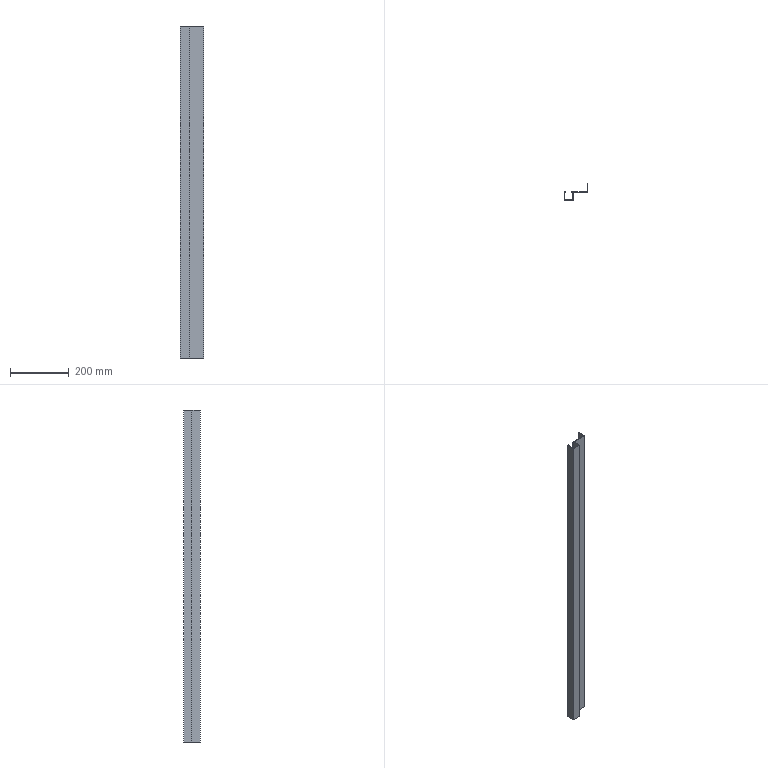Part | STEP file | Rieles_1-24 | 1 solid | 18 faces | box 81.4 x 57.7 x 1129 mm | volume 294161 mm3 | plane 18
STEP:
#1=CARTESIAN_POINT('',(10.,26.2,-677.));
#2=VERTEX_POINT('',#1);
#3=CARTESIAN_POINT('',(10.,27.7,-677.));
#4=VERTEX_POINT('',#3);
#5=CARTESIAN_POINT('',(10.,27.35,-677.));
#6=DIRECTION('',(0.,1.,0.));
#7=VECTOR('',#6,1000.);
#8=LINE('',#5,#7);
#9=EDGE_CURVE('',#2,#4,#8,.T.);
#10=ORIENTED_EDGE('',*,*,#9,.T.);
#11=CARTESIAN_POINT('',(64.2,27.7,-677.));
#12=VERTEX_POINT('',#11);
#13=CARTESIAN_POINT('',(25.,27.7,-677.));
#14=DIRECTION('',(1.,0.,0.));
#15=VECTOR('',#14,1000.);
#16=LINE('',#13,#15);
#17=EDGE_CURVE('',#4,#12,#16,.T.);
#18=ORIENTED_EDGE('',*,*,#17,.T.);
#19=CARTESIAN_POINT('',(64.2,56.2,-677.));
#20=VERTEX_POINT('',#19);
#21=CARTESIAN_POINT('',(64.2,27.35,-677.));
#22=DIRECTION('',(0.,1.,0.));
#23=VECTOR('',#22,1000.);
#24=LINE('',#21,#23);
#25=EDGE_CURVE('',#12,#20,#24,.T.);
#26=ORIENTED_EDGE('',*,*,#25,.T.);
#27=CARTESIAN_POINT('',(65.7,56.2,-677.));
#28=VERTEX_POINT('',#27);
#29=CARTESIAN_POINT('',(25.,56.2,-677.));
#30=DIRECTION('',(1.,0.,0.));
#31=VECTOR('',#30,1000.);
#32=LINE('',#29,#31);
#33=EDGE_CURVE('',#20,#28,#32,.T.);
#34=ORIENTED_EDGE('',*,*,#33,.T.);
#35=CARTESIAN_POINT('',(65.7,26.2,-677.));
#36=VERTEX_POINT('',#35);
#37=CARTESIAN_POINT('',(65.7,27.35,-677.));
#38=DIRECTION('',(0.,-1.,0.));
#39=VECTOR('',#38,1000.);
#40=LINE('',#37,#39);
#41=EDGE_CURVE('',#28,#36,#40,.T.);
#42=ORIENTED_EDGE('',*,*,#41,.T.);
#43=CARTESIAN_POINT('',(15.7,26.2,-677.));
#44=VERTEX_POINT('',#43);
#45=CARTESIAN_POINT('',(25.,26.2,-677.));
#46=DIRECTION('',(-1.,0.,0.));
#47=VECTOR('',#46,1000.);
#48=LINE('',#45,#47);
#49=EDGE_CURVE('',#36,#44,#48,.T.);
#50=ORIENTED_EDGE('',*,*,#49,.T.);
#51=CARTESIAN_POINT('',(15.7,-1.5,-677.));
#52=VERTEX_POINT('',#51);
#53=CARTESIAN_POINT('',(15.7,27.35,-677.));
#54=DIRECTION('',(0.,-1.,0.));
#55=VECTOR('',#54,1000.);
#56=LINE('',#53,#55);
#57=EDGE_CURVE('',#44,#52,#56,.T.);
#58=ORIENTED_EDGE('',*,*,#57,.T.);
#59=CARTESIAN_POINT('',(-15.7,-1.5,-677.));
#60=VERTEX_POINT('',#59);
#61=CARTESIAN_POINT('',(25.,-1.5,-677.));
#62=DIRECTION('',(-1.,0.,0.));
#63=VECTOR('',#62,1000.);
#64=LINE('',#61,#63);
#65=EDGE_CURVE('',#52,#60,#64,.T.);
#66=ORIENTED_EDGE('',*,*,#65,.T.);
#67=CARTESIAN_POINT('',(-15.7,27.7,-677.));
#68=VERTEX_POINT('',#67);
#69=CARTESIAN_POINT('',(-15.7,27.35,-677.));
#70=DIRECTION('',(0.,1.,0.));
#71=VECTOR('',#70,1000.);
#72=LINE('',#69,#71);
#73=EDGE_CURVE('',#60,#68,#72,.T.);
#74=ORIENTED_EDGE('',*,*,#73,.T.);
#75=CARTESIAN_POINT('',(-10.,27.7,-677.));
#76=VERTEX_POINT('',#75);
#77=CARTESIAN_POINT('',(25.,27.7,-677.));
#78=DIRECTION('',(1.,0.,0.));
#79=VECTOR('',#78,1000.);
#80=LINE('',#77,#79);
#81=EDGE_CURVE('',#68,#76,#80,.T.);
#82=ORIENTED_EDGE('',*,*,#81,.T.);
#83=CARTESIAN_POINT('',(-10.,26.2,-677.));
#84=VERTEX_POINT('',#83);
#85=CARTESIAN_POINT('',(-10.,27.35,-677.));
#86=DIRECTION('',(0.,-1.,0.));
#87=VECTOR('',#86,1000.);
#88=LINE('',#85,#87);
#89=EDGE_CURVE('',#76,#84,#88,.T.);
#90=ORIENTED_EDGE('',*,*,#89,.T.);
#91=CARTESIAN_POINT('',(-14.2,26.2,-677.));
#92=VERTEX_POINT('',#91);
#93=CARTESIAN_POINT('',(25.,26.2,-677.));
#94=DIRECTION('',(-1.,0.,0.));
#95=VECTOR('',#94,1000.);
#96=LINE('',#93,#95);
#97=EDGE_CURVE('',#84,#92,#96,.T.);
#98=ORIENTED_EDGE('',*,*,#97,.T.);
#99=CARTESIAN_POINT('',(-14.2,0.,-677.));
#100=VERTEX_POINT('',#99);
#101=CARTESIAN_POINT('',(-14.2,27.35,-677.));
#102=DIRECTION('',(0.,-1.,0.));
#103=VECTOR('',#102,1000.);
#104=LINE('',#101,#103);
#105=EDGE_CURVE('',#92,#100,#104,.T.);
#106=ORIENTED_EDGE('',*,*,#105,.T.);
#107=CARTESIAN_POINT('',(14.2,0.,-677.));
#108=VERTEX_POINT('',#107);
#109=CARTESIAN_POINT('',(25.,0.,-677.));
#110=DIRECTION('',(1.,0.,0.));
#111=VECTOR('',#110,1000.);
#112=LINE('',#109,#111);
#113=EDGE_CURVE('',#100,#108,#112,.T.);
#114=ORIENTED_EDGE('',*,*,#113,.T.);
#115=CARTESIAN_POINT('',(14.2,26.2,-677.));
#116=VERTEX_POINT('',#115);
#117=CARTESIAN_POINT('',(14.2,27.35,-677.));
#118=DIRECTION('',(0.,1.,0.));
#119=VECTOR('',#118,1000.);
#120=LINE('',#117,#119);
#121=EDGE_CURVE('',#108,#116,#120,.T.);
#122=ORIENTED_EDGE('',*,*,#121,.T.);
#123=CARTESIAN_POINT('',(25.,26.2,-677.));
#124=DIRECTION('',(-1.,0.,0.));
#125=VECTOR('',#124,1000.);
#126=LINE('',#123,#125);
#127=EDGE_CURVE('',#116,#2,#126,.T.);
#128=ORIENTED_EDGE('',*,*,#127,.T.);
#129=EDGE_LOOP('',(#10,#18,#26,#34,#42,#50,#58,#66,#74,#82,#90,#98,#106,#114,#122,#128));
#130=FACE_OUTER_BOUND('',#129,.T.);
#131=CARTESIAN_POINT('',(25.,27.35,-677.));
#132=DIRECTION('',(0.,0.,-1.));
#133=DIRECTION('',(0.,-1.,0.));
#134=AXIS2_PLACEMENT_3D('',#131,#132,#133);
#135=PLANE('',#134);
#136=ADVANCED_FACE('',(#130),#135,.T.);
#137=CARTESIAN_POINT('',(10.,26.2,452.));
#138=VERTEX_POINT('',#137);
#139=CARTESIAN_POINT('',(10.,27.7,452.));
#140=VERTEX_POINT('',#139);
#141=CARTESIAN_POINT('',(10.,26.2,452.));
#142=DIRECTION('',(0.,1.,0.));
#143=VECTOR('',#142,1000.);
#144=LINE('',#141,#143);
#145=EDGE_CURVE('',#138,#140,#144,.T.);
#146=ORIENTED_EDGE('',*,*,#145,.F.);
#147=CARTESIAN_POINT('',(14.2,26.2,452.));
#148=VERTEX_POINT('',#147);
#149=CARTESIAN_POINT('',(14.2,26.2,452.));
#150=DIRECTION('',(-1.,0.,0.));
#151=VECTOR('',#150,1000.);
#152=LINE('',#149,#151);
#153=EDGE_CURVE('',#148,#138,#152,.T.);
#154=ORIENTED_EDGE('',*,*,#153,.F.);
#155=CARTESIAN_POINT('',(14.2,0.,452.));
#156=VERTEX_POINT('',#155);
#157=CARTESIAN_POINT('',(14.2,0.,452.));
#158=DIRECTION('',(0.,1.,0.));
#159=VECTOR('',#158,1000.);
#160=LINE('',#157,#159);
#161=EDGE_CURVE('',#156,#148,#160,.T.);
#162=ORIENTED_EDGE('',*,*,#161,.F.);
#163=CARTESIAN_POINT('',(-14.2,0.,452.));
#164=VERTEX_POINT('',#163);
#165=CARTESIAN_POINT('',(-14.2,0.,452.));
#166=DIRECTION('',(1.,0.,0.));
#167=VECTOR('',#166,1000.);
#168=LINE('',#165,#167);
#169=EDGE_CURVE('',#164,#156,#168,.T.);
#170=ORIENTED_EDGE('',*,*,#169,.F.);
#171=CARTESIAN_POINT('',(-14.2,26.2,452.));
#172=VERTEX_POINT('',#171);
#173=CARTESIAN_POINT('',(-14.2,26.2,452.));
#174=DIRECTION('',(0.,-1.,0.));
#175=VECTOR('',#174,1000.);
#176=LINE('',#173,#175);
#177=EDGE_CURVE('',#172,#164,#176,.T.);
#178=ORIENTED_EDGE('',*,*,#177,.F.);
#179=CARTESIAN_POINT('',(-10.,26.2,452.));
#180=VERTEX_POINT('',#179);
#181=CARTESIAN_POINT('',(-10.,26.2,452.));
#182=DIRECTION('',(-1.,0.,0.));
#183=VECTOR('',#182,1000.);
#184=LINE('',#181,#183);
#185=EDGE_CURVE('',#180,#172,#184,.T.);
#186=ORIENTED_EDGE('',*,*,#185,.F.);
#187=CARTESIAN_POINT('',(-10.,27.7,452.));
#188=VERTEX_POINT('',#187);
#189=CARTESIAN_POINT('',(-10.,27.7,452.));
#190=DIRECTION('',(0.,-1.,0.));
#191=VECTOR('',#190,1000.);
#192=LINE('',#189,#191);
#193=EDGE_CURVE('',#188,#180,#192,.T.);
#194=ORIENTED_EDGE('',*,*,#193,.F.);
#195=CARTESIAN_POINT('',(-15.7,27.7,452.));
#196=VERTEX_POINT('',#195);
#197=CARTESIAN_POINT('',(-15.7,27.7,452.));
#198=DIRECTION('',(1.,0.,0.));
#199=VECTOR('',#198,1000.);
#200=LINE('',#197,#199);
#201=EDGE_CURVE('',#196,#188,#200,.T.);
#202=ORIENTED_EDGE('',*,*,#201,.F.);
#203=CARTESIAN_POINT('',(-15.7,-1.5,452.));
#204=VERTEX_POINT('',#203);
#205=CARTESIAN_POINT('',(-15.7,-1.5,452.));
#206=DIRECTION('',(0.,1.,0.));
#207=VECTOR('',#206,1000.);
#208=LINE('',#205,#207);
#209=EDGE_CURVE('',#204,#196,#208,.T.);
#210=ORIENTED_EDGE('',*,*,#209,.F.);
#211=CARTESIAN_POINT('',(15.7,-1.5,452.));
#212=VERTEX_POINT('',#211);
#213=CARTESIAN_POINT('',(15.7,-1.5,452.));
#214=DIRECTION('',(-1.,0.,0.));
#215=VECTOR('',#214,1000.);
#216=LINE('',#213,#215);
#217=EDGE_CURVE('',#212,#204,#216,.T.);
#218=ORIENTED_EDGE('',*,*,#217,.F.);
#219=CARTESIAN_POINT('',(15.7,26.2,452.));
#220=VERTEX_POINT('',#219);
#221=CARTESIAN_POINT('',(15.7,26.2,452.));
#222=DIRECTION('',(0.,-1.,0.));
#223=VECTOR('',#222,1000.);
#224=LINE('',#221,#223);
#225=EDGE_CURVE('',#220,#212,#224,.T.);
#226=ORIENTED_EDGE('',*,*,#225,.F.);
#227=CARTESIAN_POINT('',(65.7,26.2,452.));
#228=VERTEX_POINT('',#227);
#229=CARTESIAN_POINT('',(65.7,26.2,452.));
#230=DIRECTION('',(-1.,0.,0.));
#231=VECTOR('',#230,1000.);
#232=LINE('',#229,#231);
#233=EDGE_CURVE('',#228,#220,#232,.T.);
#234=ORIENTED_EDGE('',*,*,#233,.F.);
#235=CARTESIAN_POINT('',(65.7,56.2,452.));
#236=VERTEX_POINT('',#235);
#237=CARTESIAN_POINT('',(65.7,56.2,452.));
#238=DIRECTION('',(0.,-1.,0.));
#239=VECTOR('',#238,1000.);
#240=LINE('',#237,#239);
#241=EDGE_CURVE('',#236,#228,#240,.T.);
#242=ORIENTED_EDGE('',*,*,#241,.F.);
#243=CARTESIAN_POINT('',(64.2,56.2,452.));
#244=VERTEX_POINT('',#243);
#245=CARTESIAN_POINT('',(64.2,56.2,452.));
#246=DIRECTION('',(1.,0.,0.));
#247=VECTOR('',#246,1000.);
#248=LINE('',#245,#247);
#249=EDGE_CURVE('',#244,#236,#248,.T.);
#250=ORIENTED_EDGE('',*,*,#249,.F.);
#251=CARTESIAN_POINT('',(64.2,27.7,452.));
#252=VERTEX_POINT('',#251);
#253=CARTESIAN_POINT('',(64.2,27.7,452.));
#254=DIRECTION('',(0.,1.,0.));
#255=VECTOR('',#254,1000.);
#256=LINE('',#253,#255);
#257=EDGE_CURVE('',#252,#244,#256,.T.);
#258=ORIENTED_EDGE('',*,*,#257,.F.);
#259=CARTESIAN_POINT('',(10.,27.7,452.));
#260=DIRECTION('',(1.,0.,0.));
#261=VECTOR('',#260,1000.);
#262=LINE('',#259,#261);
#263=EDGE_CURVE('',#140,#252,#262,.T.);
#264=ORIENTED_EDGE('',*,*,#263,.F.);
#265=EDGE_LOOP('',(#146,#154,#162,#170,#178,#186,#194,#202,#210,#218,#226,#234,#242,#250,#258,#264));
#266=FACE_OUTER_BOUND('',#265,.T.);
#267=CARTESIAN_POINT('',(25.,27.35,452.));
#268=DIRECTION('',(0.,0.,1.));
#269=DIRECTION('',(1.,0.,0.));
#270=AXIS2_PLACEMENT_3D('',#267,#268,#269);
#271=PLANE('',#270);
#272=ADVANCED_FACE('',(#266),#271,.T.);
#273=ORIENTED_EDGE('',*,*,#145,.T.);
#274=CARTESIAN_POINT('',(10.,27.7,407.));
#275=DIRECTION('',(0.,0.,-1.));
#276=VECTOR('',#275,1000.);
#277=LINE('',#274,#276);
#278=EDGE_CURVE('',#140,#4,#277,.T.);
#279=ORIENTED_EDGE('',*,*,#278,.T.);
#280=ORIENTED_EDGE('',*,*,#9,.F.);
#281=CARTESIAN_POINT('',(10.,26.2,407.));
#282=DIRECTION('',(0.,0.,-1.));
#283=VECTOR('',#282,1000.);
#284=LINE('',#281,#283);
#285=EDGE_CURVE('',#138,#2,#284,.T.);
#286=ORIENTED_EDGE('',*,*,#285,.F.);
#287=EDGE_LOOP('',(#273,#279,#280,#286));
#288=FACE_OUTER_BOUND('',#287,.T.);
#289=CARTESIAN_POINT('',(10.,26.2,407.));
#290=DIRECTION('',(-1.,0.,0.));
#291=DIRECTION('',(0.,0.,1.));
#292=AXIS2_PLACEMENT_3D('',#289,#290,#291);
#293=PLANE('',#292);
#294=ADVANCED_FACE('',(#288),#293,.T.);
#295=ORIENTED_EDGE('',*,*,#263,.T.);
#296=CARTESIAN_POINT('',(64.2,27.7,407.));
#297=DIRECTION('',(0.,0.,-1.));
#298=VECTOR('',#297,1000.);
#299=LINE('',#296,#298);
#300=EDGE_CURVE('',#252,#12,#299,.T.);
#301=ORIENTED_EDGE('',*,*,#300,.T.);
#302=ORIENTED_EDGE('',*,*,#17,.F.);
#303=ORIENTED_EDGE('',*,*,#278,.F.);
#304=EDGE_LOOP('',(#295,#301,#302,#303));
#305=FACE_OUTER_BOUND('',#304,.T.);
#306=CARTESIAN_POINT('',(10.,27.7,407.));
#307=DIRECTION('',(0.,1.,0.));
#308=DIRECTION('',(1.,0.,0.));
#309=AXIS2_PLACEMENT_3D('',#306,#307,#308);
#310=PLANE('',#309);
#311=ADVANCED_FACE('',(#305),#310,.T.);
#312=ORIENTED_EDGE('',*,*,#257,.T.);
#313=CARTESIAN_POINT('',(64.2,56.2,407.));
#314=DIRECTION('',(0.,0.,-1.));
#315=VECTOR('',#314,1000.);
#316=LINE('',#313,#315);
#317=EDGE_CURVE('',#244,#20,#316,.T.);
#318=ORIENTED_EDGE('',*,*,#317,.T.);
#319=ORIENTED_EDGE('',*,*,#25,.F.);
#320=ORIENTED_EDGE('',*,*,#300,.F.);
#321=EDGE_LOOP('',(#312,#318,#319,#320));
#322=FACE_OUTER_BOUND('',#321,.T.);
#323=CARTESIAN_POINT('',(64.2,27.7,407.));
#324=DIRECTION('',(-1.,0.,0.));
#325=DIRECTION('',(0.,0.,1.));
#326=AXIS2_PLACEMENT_3D('',#323,#324,#325);
#327=PLANE('',#326);
#328=ADVANCED_FACE('',(#322),#327,.T.);
#329=ORIENTED_EDGE('',*,*,#249,.T.);
#330=CARTESIAN_POINT('',(65.7,56.2,407.));
#331=DIRECTION('',(0.,0.,-1.));
#332=VECTOR('',#331,1000.);
#333=LINE('',#330,#332);
#334=EDGE_CURVE('',#236,#28,#333,.T.);
#335=ORIENTED_EDGE('',*,*,#334,.T.);
#336=ORIENTED_EDGE('',*,*,#33,.F.);
#337=ORIENTED_EDGE('',*,*,#317,.F.);
#338=EDGE_LOOP('',(#329,#335,#336,#337));
#339=FACE_OUTER_BOUND('',#338,.T.);
#340=CARTESIAN_POINT('',(64.2,56.2,407.));
#341=DIRECTION('',(0.,1.,0.));
#342=DIRECTION('',(1.,0.,0.));
#343=AXIS2_PLACEMENT_3D('',#340,#341,#342);
#344=PLANE('',#343);
#345=ADVANCED_FACE('',(#339),#344,.T.);
#346=ORIENTED_EDGE('',*,*,#241,.T.);
#347=CARTESIAN_POINT('',(65.7,26.2,407.));
#348=DIRECTION('',(0.,0.,-1.));
#349=VECTOR('',#348,1000.);
#350=LINE('',#347,#349);
#351=EDGE_CURVE('',#228,#36,#350,.T.);
#352=ORIENTED_EDGE('',*,*,#351,.T.);
#353=ORIENTED_EDGE('',*,*,#41,.F.);
#354=ORIENTED_EDGE('',*,*,#334,.F.);
#355=EDGE_LOOP('',(#346,#352,#353,#354));
#356=FACE_OUTER_BOUND('',#355,.T.);
#357=CARTESIAN_POINT('',(65.7,56.2,407.));
#358=DIRECTION('',(1.,0.,0.));
#359=DIRECTION('',(0.,-1.,0.));
#360=AXIS2_PLACEMENT_3D('',#357,#358,#359);
#361=PLANE('',#360);
#362=ADVANCED_FACE('',(#356),#361,.T.);
#363=ORIENTED_EDGE('',*,*,#233,.T.);
#364=CARTESIAN_POINT('',(15.7,26.2,407.));
#365=DIRECTION('',(0.,0.,-1.));
#366=VECTOR('',#365,1000.);
#367=LINE('',#364,#366);
#368=EDGE_CURVE('',#220,#44,#367,.T.);
#369=ORIENTED_EDGE('',*,*,#368,.T.);
#370=ORIENTED_EDGE('',*,*,#49,.F.);
#371=ORIENTED_EDGE('',*,*,#351,.F.);
#372=EDGE_LOOP('',(#363,#369,#370,#371));
#373=FACE_OUTER_BOUND('',#372,.T.);
#374=CARTESIAN_POINT('',(65.7,26.2,407.));
#375=DIRECTION('',(0.,-1.,0.));
#376=DIRECTION('',(0.,0.,-1.));
#377=AXIS2_PLACEMENT_3D('',#374,#375,#376);
#378=PLANE('',#377);
#379=ADVANCED_FACE('',(#373),#378,.T.);
#380=ORIENTED_EDGE('',*,*,#225,.T.);
#381=CARTESIAN_POINT('',(15.7,-1.5,407.));
#382=DIRECTION('',(0.,0.,-1.));
#383=VECTOR('',#382,1000.);
#384=LINE('',#381,#383);
#385=EDGE_CURVE('',#212,#52,#384,.T.);
#386=ORIENTED_EDGE('',*,*,#385,.T.);
#387=ORIENTED_EDGE('',*,*,#57,.F.);
#388=ORIENTED_EDGE('',*,*,#368,.F.);
#389=EDGE_LOOP('',(#380,#386,#387,#388));
#390=FACE_OUTER_BOUND('',#389,.T.);
#391=CARTESIAN_POINT('',(15.7,26.2,407.));
#392=DIRECTION('',(1.,0.,0.));
#393=DIRECTION('',(0.,1.,0.));
#394=AXIS2_PLACEMENT_3D('',#391,#392,#393);
#395=PLANE('',#394);
#396=ADVANCED_FACE('',(#390),#395,.T.);
#397=ORIENTED_EDGE('',*,*,#217,.T.);
#398=CARTESIAN_POINT('',(-15.7,-1.5,407.));
#399=DIRECTION('',(0.,0.,-1.));
#400=VECTOR('',#399,1000.);
#401=LINE('',#398,#400);
#402=EDGE_CURVE('',#204,#60,#401,.T.);
#403=ORIENTED_EDGE('',*,*,#402,.T.);
#404=ORIENTED_EDGE('',*,*,#65,.F.);
#405=ORIENTED_EDGE('',*,*,#385,.F.);
#406=EDGE_LOOP('',(#397,#403,#404,#405));
#407=FACE_OUTER_BOUND('',#406,.T.);
#408=CARTESIAN_POINT('',(15.7,-1.5,407.));
#409=DIRECTION('',(0.,-1.,0.));
#410=DIRECTION('',(0.,0.,-1.));
#411=AXIS2_PLACEMENT_3D('',#408,#409,#410);
#412=PLANE('',#411);
#413=ADVANCED_FACE('',(#407),#412,.T.);
#414=ORIENTED_EDGE('',*,*,#209,.T.);
#415=CARTESIAN_POINT('',(-15.7,27.7,407.));
#416=DIRECTION('',(0.,0.,-1.));
#417=VECTOR('',#416,1000.);
#418=LINE('',#415,#417);
#419=EDGE_CURVE('',#196,#68,#418,.T.);
#420=ORIENTED_EDGE('',*,*,#419,.T.);
#421=ORIENTED_EDGE('',*,*,#73,.F.);
#422=ORIENTED_EDGE('',*,*,#402,.F.);
#423=EDGE_LOOP('',(#414,#420,#421,#422));
#424=FACE_OUTER_BOUND('',#423,.T.);
#425=CARTESIAN_POINT('',(-15.7,-1.5,407.));
#426=DIRECTION('',(-1.,0.,0.));
#427=DIRECTION('',(0.,0.,1.));
#428=AXIS2_PLACEMENT_3D('',#425,#426,#427);
#429=PLANE('',#428);
#430=ADVANCED_FACE('',(#424),#429,.T.);
#431=ORIENTED_EDGE('',*,*,#201,.T.);
#432=CARTESIAN_POINT('',(-10.,27.7,407.));
#433=DIRECTION('',(0.,0.,-1.));
#434=VECTOR('',#433,1000.);
#435=LINE('',#432,#434);
#436=EDGE_CURVE('',#188,#76,#435,.T.);
#437=ORIENTED_EDGE('',*,*,#436,.T.);
#438=ORIENTED_EDGE('',*,*,#81,.F.);
#439=ORIENTED_EDGE('',*,*,#419,.F.);
#440=EDGE_LOOP('',(#431,#437,#438,#439));
#441=FACE_OUTER_BOUND('',#440,.T.);
#442=CARTESIAN_POINT('',(-15.7,27.7,407.));
#443=DIRECTION('',(0.,1.,0.));
#444=DIRECTION('',(1.,0.,0.));
#445=AXIS2_PLACEMENT_3D('',#442,#443,#444);
#446=PLANE('',#445);
#447=ADVANCED_FACE('',(#441),#446,.T.);
#448=ORIENTED_EDGE('',*,*,#193,.T.);
#449=CARTESIAN_POINT('',(-10.,26.2,407.));
#450=DIRECTION('',(0.,0.,-1.));
#451=VECTOR('',#450,1000.);
#452=LINE('',#449,#451);
#453=EDGE_CURVE('',#180,#84,#452,.T.);
#454=ORIENTED_EDGE('',*,*,#453,.T.);
#455=ORIENTED_EDGE('',*,*,#89,.F.);
#456=ORIENTED_EDGE('',*,*,#436,.F.);
#457=EDGE_LOOP('',(#448,#454,#455,#456));
#458=FACE_OUTER_BOUND('',#457,.T.);
#459=CARTESIAN_POINT('',(-10.,27.7,407.));
#460=DIRECTION('',(1.,0.,0.));
#461=DIRECTION('',(0.,1.,0.));
#462=AXIS2_PLACEMENT_3D('',#459,#460,#461);
#463=PLANE('',#462);
#464=ADVANCED_FACE('',(#458),#463,.T.);
#465=ORIENTED_EDGE('',*,*,#185,.T.);
#466=CARTESIAN_POINT('',(-14.2,26.2,407.));
#467=DIRECTION('',(0.,0.,-1.));
#468=VECTOR('',#467,1000.);
#469=LINE('',#466,#468);
#470=EDGE_CURVE('',#172,#92,#469,.T.);
#471=ORIENTED_EDGE('',*,*,#470,.T.);
#472=ORIENTED_EDGE('',*,*,#97,.F.);
#473=ORIENTED_EDGE('',*,*,#453,.F.);
#474=EDGE_LOOP('',(#465,#471,#472,#473));
#475=FACE_OUTER_BOUND('',#474,.T.);
#476=CARTESIAN_POINT('',(-10.,26.2,407.));
#477=DIRECTION('',(0.,-1.,0.));
#478=DIRECTION('',(0.,0.,-1.));
#479=AXIS2_PLACEMENT_3D('',#476,#477,#478);
#480=PLANE('',#479);
#481=ADVANCED_FACE('',(#475),#480,.T.);
#482=ORIENTED_EDGE('',*,*,#177,.T.);
#483=CARTESIAN_POINT('',(-14.2,0.,407.));
#484=DIRECTION('',(0.,0.,-1.));
#485=VECTOR('',#484,1000.);
#486=LINE('',#483,#485);
#487=EDGE_CURVE('',#164,#100,#486,.T.);
#488=ORIENTED_EDGE('',*,*,#487,.T.);
#489=ORIENTED_EDGE('',*,*,#105,.F.);
#490=ORIENTED_EDGE('',*,*,#470,.F.);
#491=EDGE_LOOP('',(#482,#488,#489,#490));
#492=FACE_OUTER_BOUND('',#491,.T.);
#493=CARTESIAN_POINT('',(-14.2,26.2,407.));
#494=DIRECTION('',(1.,0.,0.));
#495=DIRECTION('',(0.,1.,0.));
#496=AXIS2_PLACEMENT_3D('',#493,#494,#495);
#497=PLANE('',#496);
#498=ADVANCED_FACE('',(#492),#497,.T.);
#499=ORIENTED_EDGE('',*,*,#169,.T.);
#500=CARTESIAN_POINT('',(14.2,0.,407.));
#501=DIRECTION('',(0.,0.,-1.));
#502=VECTOR('',#501,1000.);
#503=LINE('',#500,#502);
#504=EDGE_CURVE('',#156,#108,#503,.T.);
#505=ORIENTED_EDGE('',*,*,#504,.T.);
#506=ORIENTED_EDGE('',*,*,#113,.F.);
#507=ORIENTED_EDGE('',*,*,#487,.F.);
#508=EDGE_LOOP('',(#499,#505,#506,#507));
#509=FACE_OUTER_BOUND('',#508,.T.);
#510=CARTESIAN_POINT('',(-14.2,0.,407.));
#511=DIRECTION('',(0.,1.,0.));
#512=DIRECTION('',(1.,0.,0.));
#513=AXIS2_PLACEMENT_3D('',#510,#511,#512);
#514=PLANE('',#513);
#515=ADVANCED_FACE('',(#509),#514,.T.);
#516=ORIENTED_EDGE('',*,*,#161,.T.);
#517=CARTESIAN_POINT('',(14.2,26.2,407.));
#518=DIRECTION('',(0.,0.,-1.));
#519=VECTOR('',#518,1000.);
#520=LINE('',#517,#519);
#521=EDGE_CURVE('',#148,#116,#520,.T.);
#522=ORIENTED_EDGE('',*,*,#521,.T.);
#523=ORIENTED_EDGE('',*,*,#121,.F.);
#524=ORIENTED_EDGE('',*,*,#504,.F.);
#525=EDGE_LOOP('',(#516,#522,#523,#524));
#526=FACE_OUTER_BOUND('',#525,.T.);
#527=CARTESIAN_POINT('',(14.2,0.,407.));
#528=DIRECTION('',(-1.,0.,0.));
#529=DIRECTION('',(0.,0.,1.));
#530=AXIS2_PLACEMENT_3D('',#527,#528,#529);
#531=PLANE('',#530);
#532=ADVANCED_FACE('',(#526),#531,.T.);
#533=ORIENTED_EDGE('',*,*,#153,.T.);
#534=ORIENTED_EDGE('',*,*,#285,.T.);
#535=ORIENTED_EDGE('',*,*,#127,.F.);
#536=ORIENTED_EDGE('',*,*,#521,.F.);
#537=EDGE_LOOP('',(#533,#534,#535,#536));
#538=FACE_OUTER_BOUND('',#537,.T.);
#539=CARTESIAN_POINT('',(14.2,26.2,407.));
#540=DIRECTION('',(0.,-1.,0.));
#541=DIRECTION('',(-1.,0.,0.));
#542=AXIS2_PLACEMENT_3D('',#539,#540,#541);
#543=PLANE('',#542);
#544=ADVANCED_FACE('',(#538),#543,.T.);
#545=CLOSED_SHELL('',(#136,#272,#294,#311,#328,#345,#362,#379,#396,#413,#430,#447,#464,#481,#498,#515,#532,#544));
#546=MANIFOLD_SOLID_BREP('',#545);
#547=CARTESIAN_POINT('',(0.,0.,0.));
#548=DIRECTION('',(0.,0.,1.));
#549=DIRECTION('',(1.,0.,0.));
#550=AXIS2_PLACEMENT_3D('',#547,#548,#549);
#551=(LENGTH_UNIT()NAMED_UNIT(*)SI_UNIT(.MILLI.,.METRE.));
#552=UNCERTAINTY_MEASURE_WITH_UNIT(LENGTH_MEASURE(0.00001),#551,'','');
#553=(NAMED_UNIT(*)PLANE_ANGLE_UNIT()SI_UNIT($,.RADIAN.));
#554=(NAMED_UNIT(*)SI_UNIT($,.STERADIAN.)SOLID_ANGLE_UNIT());
#555=(GEOMETRIC_REPRESENTATION_CONTEXT(3)GLOBAL_UNCERTAINTY_ASSIGNED_CONTEXT((#552))GLOBAL_UNIT_ASSIGNED_CONTEXT((#551,#553,#554))REPRESENTATION_CONTEXT('',''));
#556=ADVANCED_BREP_SHAPE_REPRESENTATION('',(#546,#550),#555);